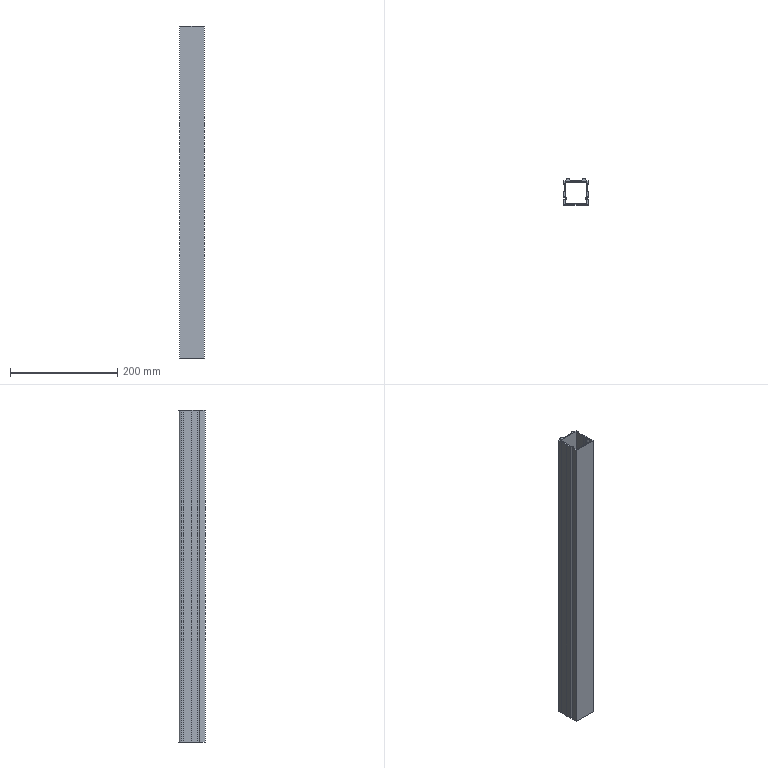Part | STEP file | MJ45 slide rail | 1 solid | 40 faces | box 45 x 49 x 620 mm | volume 255112 mm3 | plane 32 | cylinder 8 | commonest cylinder face diameters 5 x3 9 x3 8 x2
STEP:
#1=CARTESIAN_POINT('',(20.5,-14.031,310.));
#2=VERTEX_POINT('',#1);
#3=CARTESIAN_POINT('',(18.,-10.,310.));
#4=VERTEX_POINT('',#3);
#5=CARTESIAN_POINT('',(22.5,-10.,310.));
#6=DIRECTION('',(0.,0.,-1.));
#7=DIRECTION('',(1.,0.,0.));
#8=AXIS2_PLACEMENT_3D('',#5,#6,#7);
#9=CIRCLE('',#8,4.5);
#10=EDGE_CURVE('',#2,#4,#9,.T.);
#11=ORIENTED_EDGE('',*,*,#10,.T.);
#12=CARTESIAN_POINT('',(18.,-10.,-310.));
#13=VERTEX_POINT('',#12);
#14=CARTESIAN_POINT('',(18.,-10.,310.));
#15=DIRECTION('',(0.,0.,-1.));
#16=VECTOR('',#15,1000.);
#17=LINE('',#14,#16);
#18=EDGE_CURVE('',#4,#13,#17,.T.);
#19=ORIENTED_EDGE('',*,*,#18,.T.);
#20=CARTESIAN_POINT('',(20.5,-14.031,-310.));
#21=VERTEX_POINT('',#20);
#22=CARTESIAN_POINT('',(22.5,-10.,-310.));
#23=DIRECTION('',(0.,0.,-1.));
#24=DIRECTION('',(1.,0.,0.));
#25=AXIS2_PLACEMENT_3D('',#22,#23,#24);
#26=CIRCLE('',#25,4.5);
#27=EDGE_CURVE('',#21,#13,#26,.T.);
#28=ORIENTED_EDGE('',*,*,#27,.F.);
#29=CARTESIAN_POINT('',(20.5,-14.031,310.));
#30=DIRECTION('',(0.,0.,-1.));
#31=VECTOR('',#30,1000.);
#32=LINE('',#29,#31);
#33=EDGE_CURVE('',#2,#21,#32,.T.);
#34=ORIENTED_EDGE('',*,*,#33,.F.);
#35=EDGE_LOOP('',(#11,#19,#28,#34));
#36=FACE_OUTER_BOUND('',#35,.T.);
#37=CARTESIAN_POINT('',(22.5,-10.,310.));
#38=DIRECTION('',(0.,0.,-1.));
#39=DIRECTION('',(-1.,0.,0.));
#40=AXIS2_PLACEMENT_3D('',#37,#38,#39);
#41=CYLINDRICAL_SURFACE('',#40,4.5);
#42=ADVANCED_FACE('',(#36),#41,.T.);
#43=CARTESIAN_POINT('',(20.,-10.,310.));
#44=VERTEX_POINT('',#43);
#45=CARTESIAN_POINT('',(22.5,-7.5,310.));
#46=VERTEX_POINT('',#45);
#47=CARTESIAN_POINT('',(22.5,-10.,310.));
#48=DIRECTION('',(0.,0.,-1.));
#49=DIRECTION('',(1.,0.,0.));
#50=AXIS2_PLACEMENT_3D('',#47,#48,#49);
#51=CIRCLE('',#50,2.5);
#52=EDGE_CURVE('',#44,#46,#51,.T.);
#53=ORIENTED_EDGE('',*,*,#52,.F.);
#54=CARTESIAN_POINT('',(20.,-10.,-310.));
#55=VERTEX_POINT('',#54);
#56=CARTESIAN_POINT('',(20.,-10.,310.));
#57=DIRECTION('',(0.,0.,-1.));
#58=VECTOR('',#57,1000.);
#59=LINE('',#56,#58);
#60=EDGE_CURVE('',#44,#55,#59,.T.);
#61=ORIENTED_EDGE('',*,*,#60,.T.);
#62=CARTESIAN_POINT('',(22.5,-7.5,-310.));
#63=VERTEX_POINT('',#62);
#64=CARTESIAN_POINT('',(22.5,-10.,-310.));
#65=DIRECTION('',(0.,0.,-1.));
#66=DIRECTION('',(1.,0.,0.));
#67=AXIS2_PLACEMENT_3D('',#64,#65,#66);
#68=CIRCLE('',#67,2.5);
#69=EDGE_CURVE('',#55,#63,#68,.T.);
#70=ORIENTED_EDGE('',*,*,#69,.T.);
#71=CARTESIAN_POINT('',(22.5,-7.5,310.));
#72=DIRECTION('',(0.,0.,-1.));
#73=VECTOR('',#72,1000.);
#74=LINE('',#71,#73);
#75=EDGE_CURVE('',#46,#63,#74,.T.);
#76=ORIENTED_EDGE('',*,*,#75,.F.);
#77=EDGE_LOOP('',(#53,#61,#70,#76));
#78=FACE_OUTER_BOUND('',#77,.T.);
#79=CARTESIAN_POINT('',(22.5,-10.,310.));
#80=DIRECTION('',(0.,0.,-1.));
#81=DIRECTION('',(-1.,0.,0.));
#82=AXIS2_PLACEMENT_3D('',#79,#80,#81);
#83=CYLINDRICAL_SURFACE('',#82,2.5);
#84=ADVANCED_FACE('',(#78),#83,.F.);
#85=CARTESIAN_POINT('',(22.5,22.5,-310.));
#86=VERTEX_POINT('',#85);
#87=CARTESIAN_POINT('',(19.,22.5,-310.));
#88=VERTEX_POINT('',#87);
#89=CARTESIAN_POINT('',(19.,22.5,-310.));
#90=DIRECTION('',(-1.,0.,0.));
#91=VECTOR('',#90,1000.);
#92=LINE('',#89,#91);
#93=EDGE_CURVE('',#86,#88,#92,.T.);
#94=ORIENTED_EDGE('',*,*,#93,.T.);
#95=CARTESIAN_POINT('',(19.,22.5,310.));
#96=VERTEX_POINT('',#95);
#97=CARTESIAN_POINT('',(19.,22.5,310.));
#98=DIRECTION('',(0.,0.,-1.));
#99=VECTOR('',#98,1000.);
#100=LINE('',#97,#99);
#101=EDGE_CURVE('',#96,#88,#100,.T.);
#102=ORIENTED_EDGE('',*,*,#101,.F.);
#103=CARTESIAN_POINT('',(22.5,22.5,310.));
#104=VERTEX_POINT('',#103);
#105=CARTESIAN_POINT('',(19.,22.5,310.));
#106=DIRECTION('',(-1.,0.,0.));
#107=VECTOR('',#106,1000.);
#108=LINE('',#105,#107);
#109=EDGE_CURVE('',#104,#96,#108,.T.);
#110=ORIENTED_EDGE('',*,*,#109,.F.);
#111=CARTESIAN_POINT('',(22.5,22.5,310.));
#112=DIRECTION('',(0.,0.,-1.));
#113=VECTOR('',#112,1000.);
#114=LINE('',#111,#113);
#115=EDGE_CURVE('',#104,#86,#114,.T.);
#116=ORIENTED_EDGE('',*,*,#115,.T.);
#117=EDGE_LOOP('',(#94,#102,#110,#116));
#118=FACE_OUTER_BOUND('',#117,.T.);
#119=CARTESIAN_POINT('',(19.,22.5,310.));
#120=DIRECTION('',(0.,-1.,0.));
#121=DIRECTION('',(0.,0.,-1.));
#122=AXIS2_PLACEMENT_3D('',#119,#120,#121);
#123=PLANE('',#122);
#124=ADVANCED_FACE('',(#118),#123,.F.);
#125=CARTESIAN_POINT('',(11.,22.5,-310.));
#126=VERTEX_POINT('',#125);
#127=CARTESIAN_POINT('',(15.,22.5,-310.));
#128=DIRECTION('',(0.,0.,1.));
#129=DIRECTION('',(1.,0.,0.));
#130=AXIS2_PLACEMENT_3D('',#127,#128,#129);
#131=CIRCLE('',#130,4.);
#132=EDGE_CURVE('',#88,#126,#131,.T.);
#133=ORIENTED_EDGE('',*,*,#132,.T.);
#134=CARTESIAN_POINT('',(11.,22.5,310.));
#135=VERTEX_POINT('',#134);
#136=CARTESIAN_POINT('',(11.,22.5,310.));
#137=DIRECTION('',(0.,0.,-1.));
#138=VECTOR('',#137,1000.);
#139=LINE('',#136,#138);
#140=EDGE_CURVE('',#135,#126,#139,.T.);
#141=ORIENTED_EDGE('',*,*,#140,.F.);
#142=CARTESIAN_POINT('',(15.,22.5,310.));
#143=DIRECTION('',(0.,0.,1.));
#144=DIRECTION('',(1.,0.,0.));
#145=AXIS2_PLACEMENT_3D('',#142,#143,#144);
#146=CIRCLE('',#145,4.);
#147=EDGE_CURVE('',#96,#135,#146,.T.);
#148=ORIENTED_EDGE('',*,*,#147,.F.);
#149=ORIENTED_EDGE('',*,*,#101,.T.);
#150=EDGE_LOOP('',(#133,#141,#148,#149));
#151=FACE_OUTER_BOUND('',#150,.T.);
#152=CARTESIAN_POINT('',(15.,22.5,310.));
#153=DIRECTION('',(0.,0.,-1.));
#154=DIRECTION('',(-1.,0.,0.));
#155=AXIS2_PLACEMENT_3D('',#152,#153,#154);
#156=CYLINDRICAL_SURFACE('',#155,4.);
#157=ADVANCED_FACE('',(#151),#156,.T.);
#158=CARTESIAN_POINT('',(-11.,22.5,-310.));
#159=VERTEX_POINT('',#158);
#160=CARTESIAN_POINT('',(-11.,22.5,-310.));
#161=DIRECTION('',(-1.,0.,0.));
#162=VECTOR('',#161,1000.);
#163=LINE('',#160,#162);
#164=EDGE_CURVE('',#126,#159,#163,.T.);
#165=ORIENTED_EDGE('',*,*,#164,.T.);
#166=CARTESIAN_POINT('',(-11.,22.5,310.));
#167=VERTEX_POINT('',#166);
#168=CARTESIAN_POINT('',(-11.,22.5,310.));
#169=DIRECTION('',(0.,0.,-1.));
#170=VECTOR('',#169,1000.);
#171=LINE('',#168,#170);
#172=EDGE_CURVE('',#167,#159,#171,.T.);
#173=ORIENTED_EDGE('',*,*,#172,.F.);
#174=CARTESIAN_POINT('',(-11.,22.5,310.));
#175=DIRECTION('',(-1.,0.,0.));
#176=VECTOR('',#175,1000.);
#177=LINE('',#174,#176);
#178=EDGE_CURVE('',#135,#167,#177,.T.);
#179=ORIENTED_EDGE('',*,*,#178,.F.);
#180=ORIENTED_EDGE('',*,*,#140,.T.);
#181=EDGE_LOOP('',(#165,#173,#179,#180));
#182=FACE_OUTER_BOUND('',#181,.T.);
#183=CARTESIAN_POINT('',(-11.,22.5,310.));
#184=DIRECTION('',(0.,-1.,0.));
#185=DIRECTION('',(0.,0.,-1.));
#186=AXIS2_PLACEMENT_3D('',#183,#184,#185);
#187=PLANE('',#186);
#188=ADVANCED_FACE('',(#182),#187,.F.);
#189=CARTESIAN_POINT('',(-19.,22.5,-310.));
#190=VERTEX_POINT('',#189);
#191=CARTESIAN_POINT('',(-15.,22.5,-310.));
#192=DIRECTION('',(0.,0.,1.));
#193=DIRECTION('',(-1.,0.,0.));
#194=AXIS2_PLACEMENT_3D('',#191,#192,#193);
#195=CIRCLE('',#194,4.);
#196=EDGE_CURVE('',#159,#190,#195,.T.);
#197=ORIENTED_EDGE('',*,*,#196,.T.);
#198=CARTESIAN_POINT('',(-19.,22.5,310.));
#199=VERTEX_POINT('',#198);
#200=CARTESIAN_POINT('',(-19.,22.5,310.));
#201=DIRECTION('',(0.,0.,-1.));
#202=VECTOR('',#201,1000.);
#203=LINE('',#200,#202);
#204=EDGE_CURVE('',#199,#190,#203,.T.);
#205=ORIENTED_EDGE('',*,*,#204,.F.);
#206=CARTESIAN_POINT('',(-15.,22.5,310.));
#207=DIRECTION('',(0.,0.,1.));
#208=DIRECTION('',(-1.,0.,0.));
#209=AXIS2_PLACEMENT_3D('',#206,#207,#208);
#210=CIRCLE('',#209,4.);
#211=EDGE_CURVE('',#167,#199,#210,.T.);
#212=ORIENTED_EDGE('',*,*,#211,.F.);
#213=ORIENTED_EDGE('',*,*,#172,.T.);
#214=EDGE_LOOP('',(#197,#205,#212,#213));
#215=FACE_OUTER_BOUND('',#214,.T.);
#216=CARTESIAN_POINT('',(-15.,22.5,310.));
#217=DIRECTION('',(0.,0.,-1.));
#218=DIRECTION('',(-1.,0.,0.));
#219=AXIS2_PLACEMENT_3D('',#216,#217,#218);
#220=CYLINDRICAL_SURFACE('',#219,4.);
#221=ADVANCED_FACE('',(#215),#220,.T.);
#222=CARTESIAN_POINT('',(-22.5,22.5,-310.));
#223=VERTEX_POINT('',#222);
#224=CARTESIAN_POINT('',(-19.,22.5,-310.));
#225=DIRECTION('',(-1.,0.,0.));
#226=VECTOR('',#225,1000.);
#227=LINE('',#224,#226);
#228=EDGE_CURVE('',#190,#223,#227,.T.);
#229=ORIENTED_EDGE('',*,*,#228,.T.);
#230=CARTESIAN_POINT('',(-22.5,22.5,310.));
#231=VERTEX_POINT('',#230);
#232=CARTESIAN_POINT('',(-22.5,22.5,310.));
#233=DIRECTION('',(0.,0.,-1.));
#234=VECTOR('',#233,1000.);
#235=LINE('',#232,#234);
#236=EDGE_CURVE('',#231,#223,#235,.T.);
#237=ORIENTED_EDGE('',*,*,#236,.F.);
#238=CARTESIAN_POINT('',(-19.,22.5,310.));
#239=DIRECTION('',(-1.,0.,0.));
#240=VECTOR('',#239,1000.);
#241=LINE('',#238,#240);
#242=EDGE_CURVE('',#199,#231,#241,.T.);
#243=ORIENTED_EDGE('',*,*,#242,.F.);
#244=ORIENTED_EDGE('',*,*,#204,.T.);
#245=EDGE_LOOP('',(#229,#237,#243,#244));
#246=FACE_OUTER_BOUND('',#245,.T.);
#247=CARTESIAN_POINT('',(-19.,22.5,310.));
#248=DIRECTION('',(0.,-1.,0.));
#249=DIRECTION('',(1.,0.,0.));
#250=AXIS2_PLACEMENT_3D('',#247,#248,#249);
#251=PLANE('',#250);
#252=ADVANCED_FACE('',(#246),#251,.F.);
#253=CARTESIAN_POINT('',(-22.5,17.,-310.));
#254=VERTEX_POINT('',#253);
#255=CARTESIAN_POINT('',(-22.5,17.,-310.));
#256=DIRECTION('',(0.,-1.,0.));
#257=VECTOR('',#256,1000.);
#258=LINE('',#255,#257);
#259=EDGE_CURVE('',#223,#254,#258,.T.);
#260=ORIENTED_EDGE('',*,*,#259,.T.);
#261=CARTESIAN_POINT('',(-22.5,17.,310.));
#262=VERTEX_POINT('',#261);
#263=CARTESIAN_POINT('',(-22.5,17.,310.));
#264=DIRECTION('',(0.,0.,-1.));
#265=VECTOR('',#264,1000.);
#266=LINE('',#263,#265);
#267=EDGE_CURVE('',#262,#254,#266,.T.);
#268=ORIENTED_EDGE('',*,*,#267,.F.);
#269=CARTESIAN_POINT('',(-22.5,17.,310.));
#270=DIRECTION('',(0.,-1.,0.));
#271=VECTOR('',#270,1000.);
#272=LINE('',#269,#271);
#273=EDGE_CURVE('',#231,#262,#272,.T.);
#274=ORIENTED_EDGE('',*,*,#273,.F.);
#275=ORIENTED_EDGE('',*,*,#236,.T.);
#276=EDGE_LOOP('',(#260,#268,#274,#275));
#277=FACE_OUTER_BOUND('',#276,.T.);
#278=CARTESIAN_POINT('',(-22.5,17.,310.));
#279=DIRECTION('',(1.,0.,0.));
#280=DIRECTION('',(0.,1.,0.));
#281=AXIS2_PLACEMENT_3D('',#278,#279,#280);
#282=PLANE('',#281);
#283=ADVANCED_FACE('',(#277),#282,.F.);
#284=CARTESIAN_POINT('',(-21.5,17.,-310.));
#285=VERTEX_POINT('',#284);
#286=CARTESIAN_POINT('',(-21.5,17.,-310.));
#287=DIRECTION('',(1.,0.,0.));
#288=VECTOR('',#287,1000.);
#289=LINE('',#286,#288);
#290=EDGE_CURVE('',#254,#285,#289,.T.);
#291=ORIENTED_EDGE('',*,*,#290,.T.);
#292=CARTESIAN_POINT('',(-21.5,17.,310.));
#293=VERTEX_POINT('',#292);
#294=CARTESIAN_POINT('',(-21.5,17.,310.));
#295=DIRECTION('',(0.,0.,-1.));
#296=VECTOR('',#295,1000.);
#297=LINE('',#294,#296);
#298=EDGE_CURVE('',#293,#285,#297,.T.);
#299=ORIENTED_EDGE('',*,*,#298,.F.);
#300=CARTESIAN_POINT('',(-21.5,17.,310.));
#301=DIRECTION('',(1.,0.,0.));
#302=VECTOR('',#301,1000.);
#303=LINE('',#300,#302);
#304=EDGE_CURVE('',#262,#293,#303,.T.);
#305=ORIENTED_EDGE('',*,*,#304,.F.);
#306=ORIENTED_EDGE('',*,*,#267,.T.);
#307=EDGE_LOOP('',(#291,#299,#305,#306));
#308=FACE_OUTER_BOUND('',#307,.T.);
#309=CARTESIAN_POINT('',(-21.5,17.,310.));
#310=DIRECTION('',(0.,1.,0.));
#311=DIRECTION('',(0.,0.,1.));
#312=AXIS2_PLACEMENT_3D('',#309,#310,#311);
#313=PLANE('',#312);
#314=ADVANCED_FACE('',(#308),#313,.F.);
#315=CARTESIAN_POINT('',(-21.5,2.,-310.));
#316=VERTEX_POINT('',#315);
#317=CARTESIAN_POINT('',(-21.5,2.,-310.));
#318=DIRECTION('',(0.,-1.,0.));
#319=VECTOR('',#318,1000.);
#320=LINE('',#317,#319);
#321=EDGE_CURVE('',#285,#316,#320,.T.);
#322=ORIENTED_EDGE('',*,*,#321,.T.);
#323=CARTESIAN_POINT('',(-21.5,2.,310.));
#324=VERTEX_POINT('',#323);
#325=CARTESIAN_POINT('',(-21.5,2.,310.));
#326=DIRECTION('',(0.,0.,-1.));
#327=VECTOR('',#326,1000.);
#328=LINE('',#325,#327);
#329=EDGE_CURVE('',#324,#316,#328,.T.);
#330=ORIENTED_EDGE('',*,*,#329,.F.);
#331=CARTESIAN_POINT('',(-21.5,2.,310.));
#332=DIRECTION('',(0.,-1.,0.));
#333=VECTOR('',#332,1000.);
#334=LINE('',#331,#333);
#335=EDGE_CURVE('',#293,#324,#334,.T.);
#336=ORIENTED_EDGE('',*,*,#335,.F.);
#337=ORIENTED_EDGE('',*,*,#298,.T.);
#338=EDGE_LOOP('',(#322,#330,#336,#337));
#339=FACE_OUTER_BOUND('',#338,.T.);
#340=CARTESIAN_POINT('',(-21.5,2.,310.));
#341=DIRECTION('',(1.,0.,0.));
#342=DIRECTION('',(0.,0.,-1.));
#343=AXIS2_PLACEMENT_3D('',#340,#341,#342);
#344=PLANE('',#343);
#345=ADVANCED_FACE('',(#339),#344,.F.);
#346=CARTESIAN_POINT('',(-22.5,2.,-310.));
#347=VERTEX_POINT('',#346);
#348=CARTESIAN_POINT('',(-21.5,2.,-310.));
#349=DIRECTION('',(-1.,0.,0.));
#350=VECTOR('',#349,1000.);
#351=LINE('',#348,#350);
#352=EDGE_CURVE('',#316,#347,#351,.T.);
#353=ORIENTED_EDGE('',*,*,#352,.T.);
#354=CARTESIAN_POINT('',(-22.5,2.,310.));
#355=VERTEX_POINT('',#354);
#356=CARTESIAN_POINT('',(-22.5,2.,310.));
#357=DIRECTION('',(0.,0.,-1.));
#358=VECTOR('',#357,1000.);
#359=LINE('',#356,#358);
#360=EDGE_CURVE('',#355,#347,#359,.T.);
#361=ORIENTED_EDGE('',*,*,#360,.F.);
#362=CARTESIAN_POINT('',(-21.5,2.,310.));
#363=DIRECTION('',(-1.,0.,0.));
#364=VECTOR('',#363,1000.);
#365=LINE('',#362,#364);
#366=EDGE_CURVE('',#324,#355,#365,.T.);
#367=ORIENTED_EDGE('',*,*,#366,.F.);
#368=ORIENTED_EDGE('',*,*,#329,.T.);
#369=EDGE_LOOP('',(#353,#361,#367,#368));
#370=FACE_OUTER_BOUND('',#369,.T.);
#371=CARTESIAN_POINT('',(-21.5,2.,310.));
#372=DIRECTION('',(0.,-1.,0.));
#373=DIRECTION('',(0.,0.,-1.));
#374=AXIS2_PLACEMENT_3D('',#371,#372,#373);
#375=PLANE('',#374);
#376=ADVANCED_FACE('',(#370),#375,.F.);
#377=CARTESIAN_POINT('',(-22.5,-7.5,-310.));
#378=VERTEX_POINT('',#377);
#379=CARTESIAN_POINT('',(-22.5,-7.5,-310.));
#380=DIRECTION('',(0.,-1.,0.));
#381=VECTOR('',#380,1000.);
#382=LINE('',#379,#381);
#383=EDGE_CURVE('',#347,#378,#382,.T.);
#384=ORIENTED_EDGE('',*,*,#383,.T.);
#385=CARTESIAN_POINT('',(-22.5,-7.5,310.));
#386=VERTEX_POINT('',#385);
#387=CARTESIAN_POINT('',(-22.5,-7.5,310.));
#388=DIRECTION('',(0.,0.,-1.));
#389=VECTOR('',#388,1000.);
#390=LINE('',#387,#389);
#391=EDGE_CURVE('',#386,#378,#390,.T.);
#392=ORIENTED_EDGE('',*,*,#391,.F.);
#393=CARTESIAN_POINT('',(-22.5,-7.5,310.));
#394=DIRECTION('',(0.,-1.,0.));
#395=VECTOR('',#394,1000.);
#396=LINE('',#393,#395);
#397=EDGE_CURVE('',#355,#386,#396,.T.);
#398=ORIENTED_EDGE('',*,*,#397,.F.);
#399=ORIENTED_EDGE('',*,*,#360,.T.);
#400=EDGE_LOOP('',(#384,#392,#398,#399));
#401=FACE_OUTER_BOUND('',#400,.T.);
#402=CARTESIAN_POINT('',(-22.5,-7.5,310.));
#403=DIRECTION('',(1.,0.,0.));
#404=DIRECTION('',(0.,1.,0.));
#405=AXIS2_PLACEMENT_3D('',#402,#403,#404);
#406=PLANE('',#405);
#407=ADVANCED_FACE('',(#401),#406,.F.);
#408=CARTESIAN_POINT('',(-22.5,-12.5,-310.));
#409=VERTEX_POINT('',#408);
#410=CARTESIAN_POINT('',(-22.5,-10.,-310.));
#411=DIRECTION('',(0.,0.,-1.));
#412=DIRECTION('',(-1.,0.,0.));
#413=AXIS2_PLACEMENT_3D('',#410,#411,#412);
#414=CIRCLE('',#413,2.5);
#415=EDGE_CURVE('',#378,#409,#414,.T.);
#416=ORIENTED_EDGE('',*,*,#415,.T.);
#417=CARTESIAN_POINT('',(-22.5,-12.5,310.));
#418=VERTEX_POINT('',#417);
#419=CARTESIAN_POINT('',(-22.5,-12.5,310.));
#420=DIRECTION('',(0.,0.,-1.));
#421=VECTOR('',#420,1000.);
#422=LINE('',#419,#421);
#423=EDGE_CURVE('',#418,#409,#422,.T.);
#424=ORIENTED_EDGE('',*,*,#423,.F.);
#425=CARTESIAN_POINT('',(-22.5,-10.,310.));
#426=DIRECTION('',(0.,0.,-1.));
#427=DIRECTION('',(-1.,0.,0.));
#428=AXIS2_PLACEMENT_3D('',#425,#426,#427);
#429=CIRCLE('',#428,2.5);
#430=EDGE_CURVE('',#386,#418,#429,.T.);
#431=ORIENTED_EDGE('',*,*,#430,.F.);
#432=ORIENTED_EDGE('',*,*,#391,.T.);
#433=EDGE_LOOP('',(#416,#424,#431,#432));
#434=FACE_OUTER_BOUND('',#433,.T.);
#435=CARTESIAN_POINT('',(-22.5,-10.,310.));
#436=DIRECTION('',(0.,0.,-1.));
#437=DIRECTION('',(-1.,0.,0.));
#438=AXIS2_PLACEMENT_3D('',#435,#436,#437);
#439=CYLINDRICAL_SURFACE('',#438,2.5);
#440=ADVANCED_FACE('',(#434),#439,.F.);
#441=CARTESIAN_POINT('',(-22.5,-22.5,-310.));
#442=VERTEX_POINT('',#441);
#443=CARTESIAN_POINT('',(-22.5,-22.5,-310.));
#444=DIRECTION('',(0.,-1.,0.));
#445=VECTOR('',#444,1000.);
#446=LINE('',#443,#445);
#447=EDGE_CURVE('',#409,#442,#446,.T.);
#448=ORIENTED_EDGE('',*,*,#447,.T.);
#449=CARTESIAN_POINT('',(-22.5,-22.5,310.));
#450=VERTEX_POINT('',#449);
#451=CARTESIAN_POINT('',(-22.5,-22.5,310.));
#452=DIRECTION('',(0.,0.,-1.));
#453=VECTOR('',#452,1000.);
#454=LINE('',#451,#453);
#455=EDGE_CURVE('',#450,#442,#454,.T.);
#456=ORIENTED_EDGE('',*,*,#455,.F.);
#457=CARTESIAN_POINT('',(-22.5,-22.5,310.));
#458=DIRECTION('',(0.,-1.,0.));
#459=VECTOR('',#458,1000.);
#460=LINE('',#457,#459);
#461=EDGE_CURVE('',#418,#450,#460,.T.);
#462=ORIENTED_EDGE('',*,*,#461,.F.);
#463=ORIENTED_EDGE('',*,*,#423,.T.);
#464=EDGE_LOOP('',(#448,#456,#462,#463));
#465=FACE_OUTER_BOUND('',#464,.T.);
#466=CARTESIAN_POINT('',(-22.5,-22.5,310.));
#467=DIRECTION('',(1.,0.,0.));
#468=DIRECTION('',(0.,1.,0.));
#469=AXIS2_PLACEMENT_3D('',#466,#467,#468);
#470=PLANE('',#469);
#471=ADVANCED_FACE('',(#465),#470,.F.);
#472=CARTESIAN_POINT('',(22.5,-22.5,-310.));
#473=VERTEX_POINT('',#472);
#474=CARTESIAN_POINT('',(-22.5,-22.5,-310.));
#475=DIRECTION('',(1.,0.,0.));
#476=VECTOR('',#475,1000.);
#477=LINE('',#474,#476);
#478=EDGE_CURVE('',#442,#473,#477,.T.);
#479=ORIENTED_EDGE('',*,*,#478,.T.);
#480=CARTESIAN_POINT('',(22.5,-22.5,310.));
#481=VERTEX_POINT('',#480);
#482=CARTESIAN_POINT('',(22.5,-22.5,310.));
#483=DIRECTION('',(0.,0.,-1.));
#484=VECTOR('',#483,1000.);
#485=LINE('',#482,#484);
#486=EDGE_CURVE('',#481,#473,#485,.T.);
#487=ORIENTED_EDGE('',*,*,#486,.F.);
#488=CARTESIAN_POINT('',(-22.5,-22.5,310.));
#489=DIRECTION('',(1.,0.,0.));
#490=VECTOR('',#489,1000.);
#491=LINE('',#488,#490);
#492=EDGE_CURVE('',#450,#481,#491,.T.);
#493=ORIENTED_EDGE('',*,*,#492,.F.);
#494=ORIENTED_EDGE('',*,*,#455,.T.);
#495=EDGE_LOOP('',(#479,#487,#493,#494));
#496=FACE_OUTER_BOUND('',#495,.T.);
#497=CARTESIAN_POINT('',(-22.5,-22.5,310.));
#498=DIRECTION('',(0.,1.,0.));
#499=DIRECTION('',(-1.,0.,0.));
#500=AXIS2_PLACEMENT_3D('',#497,#498,#499);
#501=PLANE('',#500);
#502=ADVANCED_FACE('',(#496),#501,.F.);
#503=CARTESIAN_POINT('',(22.5,-12.5,-310.));
#504=VERTEX_POINT('',#503);
#505=CARTESIAN_POINT('',(22.5,-22.5,-310.));
#506=DIRECTION('',(0.,1.,0.));
#507=VECTOR('',#506,1000.);
#508=LINE('',#505,#507);
#509=EDGE_CURVE('',#473,#504,#508,.T.);
#510=ORIENTED_EDGE('',*,*,#509,.T.);
#511=CARTESIAN_POINT('',(22.5,-12.5,310.));
#512=VERTEX_POINT('',#511);
#513=CARTESIAN_POINT('',(22.5,-12.5,310.));
#514=DIRECTION('',(0.,0.,-1.));
#515=VECTOR('',#514,1000.);
#516=LINE('',#513,#515);
#517=EDGE_CURVE('',#512,#504,#516,.T.);
#518=ORIENTED_EDGE('',*,*,#517,.F.);
#519=CARTESIAN_POINT('',(22.5,-22.5,310.));
#520=DIRECTION('',(0.,1.,0.));
#521=VECTOR('',#520,1000.);
#522=LINE('',#519,#521);
#523=EDGE_CURVE('',#481,#512,#522,.T.);
#524=ORIENTED_EDGE('',*,*,#523,.F.);
#525=ORIENTED_EDGE('',*,*,#486,.T.);
#526=EDGE_LOOP('',(#510,#518,#524,#525));
#527=FACE_OUTER_BOUND('',#526,.T.);
#528=CARTESIAN_POINT('',(22.5,-22.5,310.));
#529=DIRECTION('',(-1.,0.,0.));
#530=DIRECTION('',(0.,-1.,0.));
#531=AXIS2_PLACEMENT_3D('',#528,#529,#530);
#532=PLANE('',#531);
#533=ADVANCED_FACE('',(#527),#532,.F.);
#534=ORIENTED_EDGE('',*,*,#60,.F.);
#535=CARTESIAN_POINT('',(22.5,-10.,310.));
#536=DIRECTION('',(0.,0.,-1.));
#537=DIRECTION('',(1.,0.,0.));
#538=AXIS2_PLACEMENT_3D('',#535,#536,#537);
#539=CIRCLE('',#538,2.5);
#540=EDGE_CURVE('',#512,#44,#539,.T.);
#541=ORIENTED_EDGE('',*,*,#540,.F.);
#542=ORIENTED_EDGE('',*,*,#517,.T.);
#543=CARTESIAN_POINT('',(22.5,-10.,-310.));
#544=DIRECTION('',(0.,0.,-1.));
#545=DIRECTION('',(1.,0.,0.));
#546=AXIS2_PLACEMENT_3D('',#543,#544,#545);
#547=CIRCLE('',#546,2.5);
#548=EDGE_CURVE('',#504,#55,#547,.T.);
#549=ORIENTED_EDGE('',*,*,#548,.T.);
#550=EDGE_LOOP('',(#534,#541,#542,#549));
#551=FACE_OUTER_BOUND('',#550,.T.);
#552=CARTESIAN_POINT('',(22.5,-10.,310.));
#553=DIRECTION('',(0.,0.,-1.));
#554=DIRECTION('',(-1.,0.,0.));
#555=AXIS2_PLACEMENT_3D('',#552,#553,#554);
#556=CYLINDRICAL_SURFACE('',#555,2.5);
#557=ADVANCED_FACE('',(#551),#556,.F.);
#558=CARTESIAN_POINT('',(22.5,2.,-310.));
#559=VERTEX_POINT('',#558);
#560=CARTESIAN_POINT('',(22.5,-7.5,-310.));
#561=DIRECTION('',(0.,1.,0.));
#562=VECTOR('',#561,1000.);
#563=LINE('',#560,#562);
#564=EDGE_CURVE('',#63,#559,#563,.T.);
#565=ORIENTED_EDGE('',*,*,#564,.T.);
#566=CARTESIAN_POINT('',(22.5,2.,310.));
#567=VERTEX_POINT('',#566);
#568=CARTESIAN_POINT('',(22.5,2.,310.));
#569=DIRECTION('',(0.,0.,-1.));
#570=VECTOR('',#569,1000.);
#571=LINE('',#568,#570);
#572=EDGE_CURVE('',#567,#559,#571,.T.);
#573=ORIENTED_EDGE('',*,*,#572,.F.);
#574=CARTESIAN_POINT('',(22.5,-7.5,310.));
#575=DIRECTION('',(0.,1.,0.));
#576=VECTOR('',#575,1000.);
#577=LINE('',#574,#576);
#578=EDGE_CURVE('',#46,#567,#577,.T.);
#579=ORIENTED_EDGE('',*,*,#578,.F.);
#580=ORIENTED_EDGE('',*,*,#75,.T.);
#581=EDGE_LOOP('',(#565,#573,#579,#580));
#582=FACE_OUTER_BOUND('',#581,.T.);
#583=CARTESIAN_POINT('',(22.5,-7.5,310.));
#584=DIRECTION('',(-1.,0.,0.));
#585=DIRECTION('',(0.,0.,1.));
#586=AXIS2_PLACEMENT_3D('',#583,#584,#585);
#587=PLANE('',#586);
#588=ADVANCED_FACE('',(#582),#587,.F.);
#589=CARTESIAN_POINT('',(21.5,2.,-310.));
#590=VERTEX_POINT('',#589);
#591=CARTESIAN_POINT('',(21.5,2.,-310.));
#592=DIRECTION('',(-1.,0.,0.));
#593=VECTOR('',#592,1000.);
#594=LINE('',#591,#593);
#595=EDGE_CURVE('',#559,#590,#594,.T.);
#596=ORIENTED_EDGE('',*,*,#595,.T.);
#597=CARTESIAN_POINT('',(21.5,2.,310.));
#598=VERTEX_POINT('',#597);
#599=CARTESIAN_POINT('',(21.5,2.,310.));
#600=DIRECTION('',(0.,0.,-1.));
#601=VECTOR('',#600,1000.);
#602=LINE('',#599,#601);
#603=EDGE_CURVE('',#598,#590,#602,.T.);
#604=ORIENTED_EDGE('',*,*,#603,.F.);
#605=CARTESIAN_POINT('',(21.5,2.,310.));
#606=DIRECTION('',(-1.,0.,0.));
#607=VECTOR('',#606,1000.);
#608=LINE('',#605,#607);
#609=EDGE_CURVE('',#567,#598,#608,.T.);
#610=ORIENTED_EDGE('',*,*,#609,.F.);
#611=ORIENTED_EDGE('',*,*,#572,.T.);
#612=EDGE_LOOP('',(#596,#604,#610,#611));
#613=FACE_OUTER_BOUND('',#612,.T.);
#614=CARTESIAN_POINT('',(21.5,2.,310.));
#615=DIRECTION('',(0.,-1.,0.));
#616=DIRECTION('',(0.,0.,-1.));
#617=AXIS2_PLACEMENT_3D('',#614,#615,#616);
#618=PLANE('',#617);
#619=ADVANCED_FACE('',(#613),#618,.F.);
#620=CARTESIAN_POINT('',(21.5,17.,-310.));
#621=VERTEX_POINT('',#620);
#622=CARTESIAN_POINT('',(21.5,2.,-310.));
#623=DIRECTION('',(0.,1.,0.));
#624=VECTOR('',#623,1000.);
#625=LINE('',#622,#624);
#626=EDGE_CURVE('',#590,#621,#625,.T.);
#627=ORIENTED_EDGE('',*,*,#626,.T.);
#628=CARTESIAN_POINT('',(21.5,17.,310.));
#629=VERTEX_POINT('',#628);
#630=CARTESIAN_POINT('',(21.5,17.,310.));
#631=DIRECTION('',(0.,0.,-1.));
#632=VECTOR('',#631,1000.);
#633=LINE('',#630,#632);
#634=EDGE_CURVE('',#629,#621,#633,.T.);
#635=ORIENTED_EDGE('',*,*,#634,.F.);
#636=CARTESIAN_POINT('',(21.5,2.,310.));
#637=DIRECTION('',(0.,1.,0.));
#638=VECTOR('',#637,1000.);
#639=LINE('',#636,#638);
#640=EDGE_CURVE('',#598,#629,#639,.T.);
#641=ORIENTED_EDGE('',*,*,#640,.F.);
#642=ORIENTED_EDGE('',*,*,#603,.T.);
#643=EDGE_LOOP('',(#627,#635,#641,#642));
#644=FACE_OUTER_BOUND('',#643,.T.);
#645=CARTESIAN_POINT('',(21.5,2.,310.));
#646=DIRECTION('',(-1.,0.,0.));
#647=DIRECTION('',(0.,0.,1.));
#648=AXIS2_PLACEMENT_3D('',#645,#646,#647);
#649=PLANE('',#648);
#650=ADVANCED_FACE('',(#644),#649,.F.);
#651=CARTESIAN_POINT('',(22.5,17.,-310.));
#652=VERTEX_POINT('',#651);
#653=CARTESIAN_POINT('',(21.5,17.,-310.));
#654=DIRECTION('',(1.,0.,0.));
#655=VECTOR('',#654,1000.);
#656=LINE('',#653,#655);
#657=EDGE_CURVE('',#621,#652,#656,.T.);
#658=ORIENTED_EDGE('',*,*,#657,.T.);
#659=CARTESIAN_POINT('',(22.5,17.,310.));
#660=VERTEX_POINT('',#659);
#661=CARTESIAN_POINT('',(22.5,17.,310.));
#662=DIRECTION('',(0.,0.,-1.));
#663=VECTOR('',#662,1000.);
#664=LINE('',#661,#663);
#665=EDGE_CURVE('',#660,#652,#664,.T.);
#666=ORIENTED_EDGE('',*,*,#665,.F.);
#667=CARTESIAN_POINT('',(21.5,17.,310.));
#668=DIRECTION('',(1.,0.,0.));
#669=VECTOR('',#668,1000.);
#670=LINE('',#667,#669);
#671=EDGE_CURVE('',#629,#660,#670,.T.);
#672=ORIENTED_EDGE('',*,*,#671,.F.);
#673=ORIENTED_EDGE('',*,*,#634,.T.);
#674=EDGE_LOOP('',(#658,#666,#672,#673));
#675=FACE_OUTER_BOUND('',#674,.T.);
#676=CARTESIAN_POINT('',(21.5,17.,310.));
#677=DIRECTION('',(0.,1.,0.));
#678=DIRECTION('',(0.,0.,1.));
#679=AXIS2_PLACEMENT_3D('',#676,#677,#678);
#680=PLANE('',#679);
#681=ADVANCED_FACE('',(#675),#680,.F.);
#682=CARTESIAN_POINT('',(22.5,17.,-310.));
#683=DIRECTION('',(0.,1.,0.));
#684=VECTOR('',#683,1000.);
#685=LINE('',#682,#684);
#686=EDGE_CURVE('',#652,#86,#685,.T.);
#687=ORIENTED_EDGE('',*,*,#686,.T.);
#688=ORIENTED_EDGE('',*,*,#115,.F.);
#689=CARTESIAN_POINT('',(22.5,17.,310.));
#690=DIRECTION('',(0.,1.,0.));
#691=VECTOR('',#690,1000.);
#692=LINE('',#689,#691);
#693=EDGE_CURVE('',#660,#104,#692,.T.);
#694=ORIENTED_EDGE('',*,*,#693,.F.);
#695=ORIENTED_EDGE('',*,*,#665,.T.);
#696=EDGE_LOOP('',(#687,#688,#694,#695));
#697=FACE_OUTER_BOUND('',#696,.T.);
#698=CARTESIAN_POINT('',(22.5,17.,310.));
#699=DIRECTION('',(-1.,0.,0.));
#700=DIRECTION('',(0.,-1.,0.));
#701=AXIS2_PLACEMENT_3D('',#698,#699,#700);
#702=PLANE('',#701);
#703=ADVANCED_FACE('',(#697),#702,.F.);
#704=CARTESIAN_POINT('',(20.5,20.5,310.));
#705=VERTEX_POINT('',#704);
#706=CARTESIAN_POINT('',(-20.5,20.5,310.));
#707=VERTEX_POINT('',#706);
#708=CARTESIAN_POINT('',(19.,20.5,310.));
#709=DIRECTION('',(-1.,0.,0.));
#710=VECTOR('',#709,1000.);
#711=LINE('',#708,#710);
#712=EDGE_CURVE('',#705,#707,#711,.T.);
#713=ORIENTED_EDGE('',*,*,#712,.F.);
#714=CARTESIAN_POINT('',(20.5,19.,310.));
#715=VERTEX_POINT('',#714);
#716=CARTESIAN_POINT('',(20.5,17.,310.));
#717=DIRECTION('',(0.,1.,0.));
#718=VECTOR('',#717,1000.);
#719=LINE('',#716,#718);
#720=EDGE_CURVE('',#715,#705,#719,.T.);
#721=ORIENTED_EDGE('',*,*,#720,.F.);
#722=CARTESIAN_POINT('',(19.5,19.,310.));
#723=VERTEX_POINT('',#722);
#724=CARTESIAN_POINT('',(21.5,19.,310.));
#725=DIRECTION('',(1.,0.,0.));
#726=VECTOR('',#725,1000.);
#727=LINE('',#724,#726);
#728=EDGE_CURVE('',#723,#715,#727,.T.);
#729=ORIENTED_EDGE('',*,*,#728,.F.);
#730=CARTESIAN_POINT('',(19.5,0.,310.));
#731=VERTEX_POINT('',#730);
#732=CARTESIAN_POINT('',(19.5,2.,310.));
#733=DIRECTION('',(0.,1.,0.));
#734=VECTOR('',#733,1000.);
#735=LINE('',#732,#734);
#736=EDGE_CURVE('',#731,#723,#735,.T.);
#737=ORIENTED_EDGE('',*,*,#736,.F.);
#738=CARTESIAN_POINT('',(20.5,0.,310.));
#739=VERTEX_POINT('',#738);
#740=CARTESIAN_POINT('',(21.5,0.,310.));
#741=DIRECTION('',(-1.,0.,0.));
#742=VECTOR('',#741,1000.);
#743=LINE('',#740,#742);
#744=EDGE_CURVE('',#739,#731,#743,.T.);
#745=ORIENTED_EDGE('',*,*,#744,.F.);
#746=CARTESIAN_POINT('',(20.5,-5.969,310.));
#747=VERTEX_POINT('',#746);
#748=CARTESIAN_POINT('',(20.5,-7.5,310.));
#749=DIRECTION('',(0.,1.,0.));
#750=VECTOR('',#749,1000.);
#751=LINE('',#748,#750);
#752=EDGE_CURVE('',#747,#739,#751,.T.);
#753=ORIENTED_EDGE('',*,*,#752,.F.);
#754=CARTESIAN_POINT('',(22.5,-10.,310.));
#755=DIRECTION('',(0.,0.,-1.));
#756=DIRECTION('',(1.,0.,0.));
#757=AXIS2_PLACEMENT_3D('',#754,#755,#756);
#758=CIRCLE('',#757,4.5);
#759=EDGE_CURVE('',#4,#747,#758,.T.);
#760=ORIENTED_EDGE('',*,*,#759,.F.);
#761=ORIENTED_EDGE('',*,*,#10,.F.);
#762=CARTESIAN_POINT('',(20.5,-20.5,310.));
#763=VERTEX_POINT('',#762);
#764=CARTESIAN_POINT('',(20.5,-22.5,310.));
#765=DIRECTION('',(0.,1.,0.));
#766=VECTOR('',#765,1000.);
#767=LINE('',#764,#766);
#768=EDGE_CURVE('',#763,#2,#767,.T.);
#769=ORIENTED_EDGE('',*,*,#768,.F.);
#770=CARTESIAN_POINT('',(-20.5,-20.5,310.));
#771=VERTEX_POINT('',#770);
#772=CARTESIAN_POINT('',(-22.5,-20.5,310.));
#773=DIRECTION('',(1.,0.,0.));
#774=VECTOR('',#773,1000.);
#775=LINE('',#772,#774);
#776=EDGE_CURVE('',#771,#763,#775,.T.);
#777=ORIENTED_EDGE('',*,*,#776,.F.);
#778=CARTESIAN_POINT('',(-20.5,-14.031,310.));
#779=VERTEX_POINT('',#778);
#780=CARTESIAN_POINT('',(-20.5,-22.5,310.));
#781=DIRECTION('',(0.,-1.,0.));
#782=VECTOR('',#781,1000.);
#783=LINE('',#780,#782);
#784=EDGE_CURVE('',#779,#771,#783,.T.);
#785=ORIENTED_EDGE('',*,*,#784,.F.);
#786=CARTESIAN_POINT('',(-20.5,-5.969,310.));
#787=VERTEX_POINT('',#786);
#788=CARTESIAN_POINT('',(-22.5,-10.,310.));
#789=DIRECTION('',(0.,0.,-1.));
#790=DIRECTION('',(1.,0.,0.));
#791=AXIS2_PLACEMENT_3D('',#788,#789,#790);
#792=CIRCLE('',#791,4.5);
#793=EDGE_CURVE('',#787,#779,#792,.T.);
#794=ORIENTED_EDGE('',*,*,#793,.F.);
#795=CARTESIAN_POINT('',(-20.5,0.,310.));
#796=VERTEX_POINT('',#795);
#797=CARTESIAN_POINT('',(-20.5,-7.5,310.));
#798=DIRECTION('',(0.,-1.,0.));
#799=VECTOR('',#798,1000.);
#800=LINE('',#797,#799);
#801=EDGE_CURVE('',#796,#787,#800,.T.);
#802=ORIENTED_EDGE('',*,*,#801,.F.);
#803=CARTESIAN_POINT('',(-19.5,0.,310.));
#804=VERTEX_POINT('',#803);
#805=CARTESIAN_POINT('',(-21.5,0.,310.));
#806=DIRECTION('',(-1.,0.,0.));
#807=VECTOR('',#806,1000.);
#808=LINE('',#805,#807);
#809=EDGE_CURVE('',#804,#796,#808,.T.);
#810=ORIENTED_EDGE('',*,*,#809,.F.);
#811=CARTESIAN_POINT('',(-19.5,19.,310.));
#812=VERTEX_POINT('',#811);
#813=CARTESIAN_POINT('',(-19.5,2.,310.));
#814=DIRECTION('',(0.,-1.,0.));
#815=VECTOR('',#814,1000.);
#816=LINE('',#813,#815);
#817=EDGE_CURVE('',#812,#804,#816,.T.);
#818=ORIENTED_EDGE('',*,*,#817,.F.);
#819=CARTESIAN_POINT('',(-20.5,19.,310.));
#820=VERTEX_POINT('',#819);
#821=CARTESIAN_POINT('',(-21.5,19.,310.));
#822=DIRECTION('',(1.,0.,0.));
#823=VECTOR('',#822,1000.);
#824=LINE('',#821,#823);
#825=EDGE_CURVE('',#820,#812,#824,.T.);
#826=ORIENTED_EDGE('',*,*,#825,.F.);
#827=CARTESIAN_POINT('',(-20.5,17.,310.));
#828=DIRECTION('',(0.,-1.,0.));
#829=VECTOR('',#828,1000.);
#830=LINE('',#827,#829);
#831=EDGE_CURVE('',#707,#820,#830,.T.);
#832=ORIENTED_EDGE('',*,*,#831,.F.);
#833=EDGE_LOOP('',(#713,#721,#729,#737,#745,#753,#760,#761,#769,#777,#785,#794,#802,#810,#818,#826,#832));
#834=FACE_BOUND('',#833,.T.);
#835=ORIENTED_EDGE('',*,*,#109,.T.);
#836=ORIENTED_EDGE('',*,*,#147,.T.);
#837=ORIENTED_EDGE('',*,*,#178,.T.);
#838=ORIENTED_EDGE('',*,*,#211,.T.);
#839=ORIENTED_EDGE('',*,*,#242,.T.);
#840=ORIENTED_EDGE('',*,*,#273,.T.);
#841=ORIENTED_EDGE('',*,*,#304,.T.);
#842=ORIENTED_EDGE('',*,*,#335,.T.);
#843=ORIENTED_EDGE('',*,*,#366,.T.);
#844=ORIENTED_EDGE('',*,*,#397,.T.);
#845=ORIENTED_EDGE('',*,*,#430,.T.);
#846=ORIENTED_EDGE('',*,*,#461,.T.);
#847=ORIENTED_EDGE('',*,*,#492,.T.);
#848=ORIENTED_EDGE('',*,*,#523,.T.);
#849=ORIENTED_EDGE('',*,*,#540,.T.);
#850=ORIENTED_EDGE('',*,*,#52,.T.);
#851=ORIENTED_EDGE('',*,*,#578,.T.);
#852=ORIENTED_EDGE('',*,*,#609,.T.);
#853=ORIENTED_EDGE('',*,*,#640,.T.);
#854=ORIENTED_EDGE('',*,*,#671,.T.);
#855=ORIENTED_EDGE('',*,*,#693,.T.);
#856=EDGE_LOOP('',(#835,#836,#837,#838,#839,#840,#841,#842,#843,#844,#845,#846,#847,#848,#849,#850,#851,#852,#853,#854,#855));
#857=FACE_OUTER_BOUND('',#856,.T.);
#858=CARTESIAN_POINT('',(22.5,-10.,310.));
#859=DIRECTION('',(0.,0.,1.));
#860=DIRECTION('',(1.,0.,0.));
#861=AXIS2_PLACEMENT_3D('',#858,#859,#860);
#862=PLANE('',#861);
#863=ADVANCED_FACE('',(#834,#857),#862,.T.);
#864=CARTESIAN_POINT('',(20.5,19.,-310.));
#865=VERTEX_POINT('',#864);
#866=CARTESIAN_POINT('',(20.5,20.5,-310.));
#867=VERTEX_POINT('',#866);
#868=CARTESIAN_POINT('',(20.5,17.,-310.));
#869=DIRECTION('',(0.,1.,0.));
#870=VECTOR('',#869,1000.);
#871=LINE('',#868,#870);
#872=EDGE_CURVE('',#865,#867,#871,.T.);
#873=ORIENTED_EDGE('',*,*,#872,.T.);
#874=CARTESIAN_POINT('',(-20.5,20.5,-310.));
#875=VERTEX_POINT('',#874);
#876=CARTESIAN_POINT('',(-19.,20.5,-310.));
#877=DIRECTION('',(-1.,0.,0.));
#878=VECTOR('',#877,1000.);
#879=LINE('',#876,#878);
#880=EDGE_CURVE('',#867,#875,#879,.T.);
#881=ORIENTED_EDGE('',*,*,#880,.T.);
#882=CARTESIAN_POINT('',(-20.5,19.,-310.));
#883=VERTEX_POINT('',#882);
#884=CARTESIAN_POINT('',(-20.5,17.,-310.));
#885=DIRECTION('',(0.,-1.,0.));
#886=VECTOR('',#885,1000.);
#887=LINE('',#884,#886);
#888=EDGE_CURVE('',#875,#883,#887,.T.);
#889=ORIENTED_EDGE('',*,*,#888,.T.);
#890=CARTESIAN_POINT('',(-19.5,19.,-310.));
#891=VERTEX_POINT('',#890);
#892=CARTESIAN_POINT('',(-21.5,19.,-310.));
#893=DIRECTION('',(1.,0.,0.));
#894=VECTOR('',#893,1000.);
#895=LINE('',#892,#894);
#896=EDGE_CURVE('',#883,#891,#895,.T.);
#897=ORIENTED_EDGE('',*,*,#896,.T.);
#898=CARTESIAN_POINT('',(-19.5,0.,-310.));
#899=VERTEX_POINT('',#898);
#900=CARTESIAN_POINT('',(-19.5,2.,-310.));
#901=DIRECTION('',(0.,-1.,0.));
#902=VECTOR('',#901,1000.);
#903=LINE('',#900,#902);
#904=EDGE_CURVE('',#891,#899,#903,.T.);
#905=ORIENTED_EDGE('',*,*,#904,.T.);
#906=CARTESIAN_POINT('',(-20.5,0.,-310.));
#907=VERTEX_POINT('',#906);
#908=CARTESIAN_POINT('',(-21.5,0.,-310.));
#909=DIRECTION('',(-1.,0.,0.));
#910=VECTOR('',#909,1000.);
#911=LINE('',#908,#910);
#912=EDGE_CURVE('',#899,#907,#911,.T.);
#913=ORIENTED_EDGE('',*,*,#912,.T.);
#914=CARTESIAN_POINT('',(-20.5,-5.969,-310.));
#915=VERTEX_POINT('',#914);
#916=CARTESIAN_POINT('',(-20.5,-7.5,-310.));
#917=DIRECTION('',(0.,-1.,0.));
#918=VECTOR('',#917,1000.);
#919=LINE('',#916,#918);
#920=EDGE_CURVE('',#907,#915,#919,.T.);
#921=ORIENTED_EDGE('',*,*,#920,.T.);
#922=CARTESIAN_POINT('',(-20.5,-14.031,-310.));
#923=VERTEX_POINT('',#922);
#924=CARTESIAN_POINT('',(-22.5,-10.,-310.));
#925=DIRECTION('',(0.,0.,-1.));
#926=DIRECTION('',(1.,0.,0.));
#927=AXIS2_PLACEMENT_3D('',#924,#925,#926);
#928=CIRCLE('',#927,4.5);
#929=EDGE_CURVE('',#915,#923,#928,.T.);
#930=ORIENTED_EDGE('',*,*,#929,.T.);
#931=CARTESIAN_POINT('',(-20.5,-20.5,-310.));
#932=VERTEX_POINT('',#931);
#933=CARTESIAN_POINT('',(-20.5,-22.5,-310.));
#934=DIRECTION('',(0.,-1.,0.));
#935=VECTOR('',#934,1000.);
#936=LINE('',#933,#935);
#937=EDGE_CURVE('',#923,#932,#936,.T.);
#938=ORIENTED_EDGE('',*,*,#937,.T.);
#939=CARTESIAN_POINT('',(20.5,-20.5,-310.));
#940=VERTEX_POINT('',#939);
#941=CARTESIAN_POINT('',(-22.5,-20.5,-310.));
#942=DIRECTION('',(1.,0.,0.));
#943=VECTOR('',#942,1000.);
#944=LINE('',#941,#943);
#945=EDGE_CURVE('',#932,#940,#944,.T.);
#946=ORIENTED_EDGE('',*,*,#945,.T.);
#947=CARTESIAN_POINT('',(20.5,-22.5,-310.));
#948=DIRECTION('',(0.,1.,0.));
#949=VECTOR('',#948,1000.);
#950=LINE('',#947,#949);
#951=EDGE_CURVE('',#940,#21,#950,.T.);
#952=ORIENTED_EDGE('',*,*,#951,.T.);
#953=ORIENTED_EDGE('',*,*,#27,.T.);
#954=CARTESIAN_POINT('',(20.5,-5.969,-310.));
#955=VERTEX_POINT('',#954);
#956=CARTESIAN_POINT('',(22.5,-10.,-310.));
#957=DIRECTION('',(0.,0.,-1.));
#958=DIRECTION('',(1.,0.,0.));
#959=AXIS2_PLACEMENT_3D('',#956,#957,#958);
#960=CIRCLE('',#959,4.5);
#961=EDGE_CURVE('',#13,#955,#960,.T.);
#962=ORIENTED_EDGE('',*,*,#961,.T.);
#963=CARTESIAN_POINT('',(20.5,0.,-310.));
#964=VERTEX_POINT('',#963);
#965=CARTESIAN_POINT('',(20.5,-7.5,-310.));
#966=DIRECTION('',(0.,1.,0.));
#967=VECTOR('',#966,1000.);
#968=LINE('',#965,#967);
#969=EDGE_CURVE('',#955,#964,#968,.T.);
#970=ORIENTED_EDGE('',*,*,#969,.T.);
#971=CARTESIAN_POINT('',(19.5,0.,-310.));
#972=VERTEX_POINT('',#971);
#973=CARTESIAN_POINT('',(21.5,0.,-310.));
#974=DIRECTION('',(-1.,0.,0.));
#975=VECTOR('',#974,1000.);
#976=LINE('',#973,#975);
#977=EDGE_CURVE('',#964,#972,#976,.T.);
#978=ORIENTED_EDGE('',*,*,#977,.T.);
#979=CARTESIAN_POINT('',(19.5,19.,-310.));
#980=VERTEX_POINT('',#979);
#981=CARTESIAN_POINT('',(19.5,2.,-310.));
#982=DIRECTION('',(0.,1.,0.));
#983=VECTOR('',#982,1000.);
#984=LINE('',#981,#983);
#985=EDGE_CURVE('',#972,#980,#984,.T.);
#986=ORIENTED_EDGE('',*,*,#985,.T.);
#987=CARTESIAN_POINT('',(21.5,19.,-310.));
#988=DIRECTION('',(1.,0.,0.));
#989=VECTOR('',#988,1000.);
#990=LINE('',#987,#989);
#991=EDGE_CURVE('',#980,#865,#990,.T.);
#992=ORIENTED_EDGE('',*,*,#991,.T.);
#993=EDGE_LOOP('',(#873,#881,#889,#897,#905,#913,#921,#930,#938,#946,#952,#953,#962,#970,#978,#986,#992));
#994=FACE_BOUND('',#993,.T.);
#995=ORIENTED_EDGE('',*,*,#93,.F.);
#996=ORIENTED_EDGE('',*,*,#686,.F.);
#997=ORIENTED_EDGE('',*,*,#657,.F.);
#998=ORIENTED_EDGE('',*,*,#626,.F.);
#999=ORIENTED_EDGE('',*,*,#595,.F.);
#1000=ORIENTED_EDGE('',*,*,#564,.F.);
#1001=ORIENTED_EDGE('',*,*,#69,.F.);
#1002=ORIENTED_EDGE('',*,*,#548,.F.);
#1003=ORIENTED_EDGE('',*,*,#509,.F.);
#1004=ORIENTED_EDGE('',*,*,#478,.F.);
#1005=ORIENTED_EDGE('',*,*,#447,.F.);
#1006=ORIENTED_EDGE('',*,*,#415,.F.);
#1007=ORIENTED_EDGE('',*,*,#383,.F.);
#1008=ORIENTED_EDGE('',*,*,#352,.F.);
#1009=ORIENTED_EDGE('',*,*,#321,.F.);
#1010=ORIENTED_EDGE('',*,*,#290,.F.);
#1011=ORIENTED_EDGE('',*,*,#259,.F.);
#1012=ORIENTED_EDGE('',*,*,#228,.F.);
#1013=ORIENTED_EDGE('',*,*,#196,.F.);
#1014=ORIENTED_EDGE('',*,*,#164,.F.);
#1015=ORIENTED_EDGE('',*,*,#132,.F.);
#1016=EDGE_LOOP('',(#995,#996,#997,#998,#999,#1000,#1001,#1002,#1003,#1004,#1005,#1006,#1007,#1008,#1009,#1010,#1011,#1012,#1013,#1014,#1015));
#1017=FACE_OUTER_BOUND('',#1016,.T.);
#1018=CARTESIAN_POINT('',(22.5,-10.,-310.));
#1019=DIRECTION('',(0.,0.,1.));
#1020=DIRECTION('',(1.,0.,0.));
#1021=AXIS2_PLACEMENT_3D('',#1018,#1019,#1020);
#1022=PLANE('',#1021);
#1023=ADVANCED_FACE('',(#994,#1017),#1022,.F.);
#1024=ORIENTED_EDGE('',*,*,#880,.F.);
#1025=CARTESIAN_POINT('',(20.5,20.5,310.));
#1026=DIRECTION('',(0.,0.,-1.));
#1027=VECTOR('',#1026,1000.);
#1028=LINE('',#1025,#1027);
#1029=EDGE_CURVE('',#705,#867,#1028,.T.);
#1030=ORIENTED_EDGE('',*,*,#1029,.F.);
#1031=ORIENTED_EDGE('',*,*,#712,.T.);
#1032=CARTESIAN_POINT('',(-20.5,20.5,310.));
#1033=DIRECTION('',(0.,0.,-1.));
#1034=VECTOR('',#1033,1000.);
#1035=LINE('',#1032,#1034);
#1036=EDGE_CURVE('',#707,#875,#1035,.T.);
#1037=ORIENTED_EDGE('',*,*,#1036,.T.);
#1038=EDGE_LOOP('',(#1024,#1030,#1031,#1037));
#1039=FACE_OUTER_BOUND('',#1038,.T.);
#1040=CARTESIAN_POINT('',(-19.,20.5,310.));
#1041=DIRECTION('',(0.,-1.,0.));
#1042=DIRECTION('',(1.,0.,0.));
#1043=AXIS2_PLACEMENT_3D('',#1040,#1041,#1042);
#1044=PLANE('',#1043);
#1045=ADVANCED_FACE('',(#1039),#1044,.T.);
#1046=ORIENTED_EDGE('',*,*,#888,.F.);
#1047=ORIENTED_EDGE('',*,*,#1036,.F.);
#1048=ORIENTED_EDGE('',*,*,#831,.T.);
#1049=CARTESIAN_POINT('',(-20.5,19.,310.));
#1050=DIRECTION('',(0.,0.,-1.));
#1051=VECTOR('',#1050,1000.);
#1052=LINE('',#1049,#1051);
#1053=EDGE_CURVE('',#820,#883,#1052,.T.);
#1054=ORIENTED_EDGE('',*,*,#1053,.T.);
#1055=EDGE_LOOP('',(#1046,#1047,#1048,#1054));
#1056=FACE_OUTER_BOUND('',#1055,.T.);
#1057=CARTESIAN_POINT('',(-20.5,17.,310.));
#1058=DIRECTION('',(1.,0.,0.));
#1059=DIRECTION('',(0.,1.,0.));
#1060=AXIS2_PLACEMENT_3D('',#1057,#1058,#1059);
#1061=PLANE('',#1060);
#1062=ADVANCED_FACE('',(#1056),#1061,.T.);
#1063=ORIENTED_EDGE('',*,*,#896,.F.);
#1064=ORIENTED_EDGE('',*,*,#1053,.F.);
#1065=ORIENTED_EDGE('',*,*,#825,.T.);
#1066=CARTESIAN_POINT('',(-19.5,19.,310.));
#1067=DIRECTION('',(0.,0.,-1.));
#1068=VECTOR('',#1067,1000.);
#1069=LINE('',#1066,#1068);
#1070=EDGE_CURVE('',#812,#891,#1069,.T.);
#1071=ORIENTED_EDGE('',*,*,#1070,.T.);
#1072=EDGE_LOOP('',(#1063,#1064,#1065,#1071));
#1073=FACE_OUTER_BOUND('',#1072,.T.);
#1074=CARTESIAN_POINT('',(-21.5,19.,310.));
#1075=DIRECTION('',(0.,1.,0.));
#1076=DIRECTION('',(0.,0.,1.));
#1077=AXIS2_PLACEMENT_3D('',#1074,#1075,#1076);
#1078=PLANE('',#1077);
#1079=ADVANCED_FACE('',(#1073),#1078,.T.);
#1080=ORIENTED_EDGE('',*,*,#904,.F.);
#1081=ORIENTED_EDGE('',*,*,#1070,.F.);
#1082=ORIENTED_EDGE('',*,*,#817,.T.);
#1083=CARTESIAN_POINT('',(-19.5,0.,310.));
#1084=DIRECTION('',(0.,0.,-1.));
#1085=VECTOR('',#1084,1000.);
#1086=LINE('',#1083,#1085);
#1087=EDGE_CURVE('',#804,#899,#1086,.T.);
#1088=ORIENTED_EDGE('',*,*,#1087,.T.);
#1089=EDGE_LOOP('',(#1080,#1081,#1082,#1088));
#1090=FACE_OUTER_BOUND('',#1089,.T.);
#1091=CARTESIAN_POINT('',(-19.5,2.,310.));
#1092=DIRECTION('',(1.,0.,0.));
#1093=DIRECTION('',(0.,0.,-1.));
#1094=AXIS2_PLACEMENT_3D('',#1091,#1092,#1093);
#1095=PLANE('',#1094);
#1096=ADVANCED_FACE('',(#1090),#1095,.T.);
#1097=ORIENTED_EDGE('',*,*,#912,.F.);
#1098=ORIENTED_EDGE('',*,*,#1087,.F.);
#1099=ORIENTED_EDGE('',*,*,#809,.T.);
#1100=CARTESIAN_POINT('',(-20.5,0.,310.));
#1101=DIRECTION('',(0.,0.,-1.));
#1102=VECTOR('',#1101,1000.);
#1103=LINE('',#1100,#1102);
#1104=EDGE_CURVE('',#796,#907,#1103,.T.);
#1105=ORIENTED_EDGE('',*,*,#1104,.T.);
#1106=EDGE_LOOP('',(#1097,#1098,#1099,#1105));
#1107=FACE_OUTER_BOUND('',#1106,.T.);
#1108=CARTESIAN_POINT('',(-21.5,0.,310.));
#1109=DIRECTION('',(0.,-1.,0.));
#1110=DIRECTION('',(0.,0.,-1.));
#1111=AXIS2_PLACEMENT_3D('',#1108,#1109,#1110);
#1112=PLANE('',#1111);
#1113=ADVANCED_FACE('',(#1107),#1112,.T.);
#1114=ORIENTED_EDGE('',*,*,#920,.F.);
#1115=ORIENTED_EDGE('',*,*,#1104,.F.);
#1116=ORIENTED_EDGE('',*,*,#801,.T.);
#1117=CARTESIAN_POINT('',(-20.5,-5.969,310.));
#1118=DIRECTION('',(0.,0.,-1.));
#1119=VECTOR('',#1118,1000.);
#1120=LINE('',#1117,#1119);
#1121=EDGE_CURVE('',#787,#915,#1120,.T.);
#1122=ORIENTED_EDGE('',*,*,#1121,.T.);
#1123=EDGE_LOOP('',(#1114,#1115,#1116,#1122));
#1124=FACE_OUTER_BOUND('',#1123,.T.);
#1125=CARTESIAN_POINT('',(-20.5,-7.5,310.));
#1126=DIRECTION('',(1.,0.,0.));
#1127=DIRECTION('',(0.,1.,0.));
#1128=AXIS2_PLACEMENT_3D('',#1125,#1126,#1127);
#1129=PLANE('',#1128);
#1130=ADVANCED_FACE('',(#1124),#1129,.T.);
#1131=ORIENTED_EDGE('',*,*,#929,.F.);
#1132=ORIENTED_EDGE('',*,*,#1121,.F.);
#1133=ORIENTED_EDGE('',*,*,#793,.T.);
#1134=CARTESIAN_POINT('',(-20.5,-14.031,310.));
#1135=DIRECTION('',(0.,0.,-1.));
#1136=VECTOR('',#1135,1000.);
#1137=LINE('',#1134,#1136);
#1138=EDGE_CURVE('',#779,#923,#1137,.T.);
#1139=ORIENTED_EDGE('',*,*,#1138,.T.);
#1140=EDGE_LOOP('',(#1131,#1132,#1133,#1139));
#1141=FACE_OUTER_BOUND('',#1140,.T.);
#1142=CARTESIAN_POINT('',(-22.5,-10.,310.));
#1143=DIRECTION('',(0.,0.,-1.));
#1144=DIRECTION('',(-1.,0.,0.));
#1145=AXIS2_PLACEMENT_3D('',#1142,#1143,#1144);
#1146=CYLINDRICAL_SURFACE('',#1145,4.5);
#1147=ADVANCED_FACE('',(#1141),#1146,.T.);
#1148=ORIENTED_EDGE('',*,*,#937,.F.);
#1149=ORIENTED_EDGE('',*,*,#1138,.F.);
#1150=ORIENTED_EDGE('',*,*,#784,.T.);
#1151=CARTESIAN_POINT('',(-20.5,-20.5,310.));
#1152=DIRECTION('',(0.,0.,-1.));
#1153=VECTOR('',#1152,1000.);
#1154=LINE('',#1151,#1153);
#1155=EDGE_CURVE('',#771,#932,#1154,.T.);
#1156=ORIENTED_EDGE('',*,*,#1155,.T.);
#1157=EDGE_LOOP('',(#1148,#1149,#1150,#1156));
#1158=FACE_OUTER_BOUND('',#1157,.T.);
#1159=CARTESIAN_POINT('',(-20.5,-22.5,310.));
#1160=DIRECTION('',(1.,0.,0.));
#1161=DIRECTION('',(0.,1.,0.));
#1162=AXIS2_PLACEMENT_3D('',#1159,#1160,#1161);
#1163=PLANE('',#1162);
#1164=ADVANCED_FACE('',(#1158),#1163,.T.);
#1165=ORIENTED_EDGE('',*,*,#945,.F.);
#1166=ORIENTED_EDGE('',*,*,#1155,.F.);
#1167=ORIENTED_EDGE('',*,*,#776,.T.);
#1168=CARTESIAN_POINT('',(20.5,-20.5,310.));
#1169=DIRECTION('',(0.,0.,-1.));
#1170=VECTOR('',#1169,1000.);
#1171=LINE('',#1168,#1170);
#1172=EDGE_CURVE('',#763,#940,#1171,.T.);
#1173=ORIENTED_EDGE('',*,*,#1172,.T.);
#1174=EDGE_LOOP('',(#1165,#1166,#1167,#1173));
#1175=FACE_OUTER_BOUND('',#1174,.T.);
#1176=CARTESIAN_POINT('',(-22.5,-20.5,310.));
#1177=DIRECTION('',(0.,1.,0.));
#1178=DIRECTION('',(-1.,0.,0.));
#1179=AXIS2_PLACEMENT_3D('',#1176,#1177,#1178);
#1180=PLANE('',#1179);
#1181=ADVANCED_FACE('',(#1175),#1180,.T.);
#1182=ORIENTED_EDGE('',*,*,#951,.F.);
#1183=ORIENTED_EDGE('',*,*,#1172,.F.);
#1184=ORIENTED_EDGE('',*,*,#768,.T.);
#1185=ORIENTED_EDGE('',*,*,#33,.T.);
#1186=EDGE_LOOP('',(#1182,#1183,#1184,#1185));
#1187=FACE_OUTER_BOUND('',#1186,.T.);
#1188=CARTESIAN_POINT('',(20.5,-22.5,310.));
#1189=DIRECTION('',(-1.,0.,0.));
#1190=DIRECTION('',(0.,-1.,0.));
#1191=AXIS2_PLACEMENT_3D('',#1188,#1189,#1190);
#1192=PLANE('',#1191);
#1193=ADVANCED_FACE('',(#1187),#1192,.T.);
#1194=ORIENTED_EDGE('',*,*,#18,.F.);
#1195=ORIENTED_EDGE('',*,*,#759,.T.);
#1196=CARTESIAN_POINT('',(20.5,-5.969,310.));
#1197=DIRECTION('',(0.,0.,-1.));
#1198=VECTOR('',#1197,1000.);
#1199=LINE('',#1196,#1198);
#1200=EDGE_CURVE('',#747,#955,#1199,.T.);
#1201=ORIENTED_EDGE('',*,*,#1200,.T.);
#1202=ORIENTED_EDGE('',*,*,#961,.F.);
#1203=EDGE_LOOP('',(#1194,#1195,#1201,#1202));
#1204=FACE_OUTER_BOUND('',#1203,.T.);
#1205=CARTESIAN_POINT('',(22.5,-10.,310.));
#1206=DIRECTION('',(0.,0.,-1.));
#1207=DIRECTION('',(-1.,0.,0.));
#1208=AXIS2_PLACEMENT_3D('',#1205,#1206,#1207);
#1209=CYLINDRICAL_SURFACE('',#1208,4.5);
#1210=ADVANCED_FACE('',(#1204),#1209,.T.);
#1211=ORIENTED_EDGE('',*,*,#969,.F.);
#1212=ORIENTED_EDGE('',*,*,#1200,.F.);
#1213=ORIENTED_EDGE('',*,*,#752,.T.);
#1214=CARTESIAN_POINT('',(20.5,0.,310.));
#1215=DIRECTION('',(0.,0.,-1.));
#1216=VECTOR('',#1215,1000.);
#1217=LINE('',#1214,#1216);
#1218=EDGE_CURVE('',#739,#964,#1217,.T.);
#1219=ORIENTED_EDGE('',*,*,#1218,.T.);
#1220=EDGE_LOOP('',(#1211,#1212,#1213,#1219));
#1221=FACE_OUTER_BOUND('',#1220,.T.);
#1222=CARTESIAN_POINT('',(20.5,-7.5,310.));
#1223=DIRECTION('',(-1.,0.,0.));
#1224=DIRECTION('',(0.,0.,1.));
#1225=AXIS2_PLACEMENT_3D('',#1222,#1223,#1224);
#1226=PLANE('',#1225);
#1227=ADVANCED_FACE('',(#1221),#1226,.T.);
#1228=ORIENTED_EDGE('',*,*,#977,.F.);
#1229=ORIENTED_EDGE('',*,*,#1218,.F.);
#1230=ORIENTED_EDGE('',*,*,#744,.T.);
#1231=CARTESIAN_POINT('',(19.5,0.,310.));
#1232=DIRECTION('',(0.,0.,-1.));
#1233=VECTOR('',#1232,1000.);
#1234=LINE('',#1231,#1233);
#1235=EDGE_CURVE('',#731,#972,#1234,.T.);
#1236=ORIENTED_EDGE('',*,*,#1235,.T.);
#1237=EDGE_LOOP('',(#1228,#1229,#1230,#1236));
#1238=FACE_OUTER_BOUND('',#1237,.T.);
#1239=CARTESIAN_POINT('',(21.5,0.,310.));
#1240=DIRECTION('',(0.,-1.,0.));
#1241=DIRECTION('',(0.,0.,-1.));
#1242=AXIS2_PLACEMENT_3D('',#1239,#1240,#1241);
#1243=PLANE('',#1242);
#1244=ADVANCED_FACE('',(#1238),#1243,.T.);
#1245=ORIENTED_EDGE('',*,*,#985,.F.);
#1246=ORIENTED_EDGE('',*,*,#1235,.F.);
#1247=ORIENTED_EDGE('',*,*,#736,.T.);
#1248=CARTESIAN_POINT('',(19.5,19.,310.));
#1249=DIRECTION('',(0.,0.,-1.));
#1250=VECTOR('',#1249,1000.);
#1251=LINE('',#1248,#1250);
#1252=EDGE_CURVE('',#723,#980,#1251,.T.);
#1253=ORIENTED_EDGE('',*,*,#1252,.T.);
#1254=EDGE_LOOP('',(#1245,#1246,#1247,#1253));
#1255=FACE_OUTER_BOUND('',#1254,.T.);
#1256=CARTESIAN_POINT('',(19.5,2.,310.));
#1257=DIRECTION('',(-1.,0.,0.));
#1258=DIRECTION('',(0.,0.,1.));
#1259=AXIS2_PLACEMENT_3D('',#1256,#1257,#1258);
#1260=PLANE('',#1259);
#1261=ADVANCED_FACE('',(#1255),#1260,.T.);
#1262=ORIENTED_EDGE('',*,*,#991,.F.);
#1263=ORIENTED_EDGE('',*,*,#1252,.F.);
#1264=ORIENTED_EDGE('',*,*,#728,.T.);
#1265=CARTESIAN_POINT('',(20.5,19.,310.));
#1266=DIRECTION('',(0.,0.,-1.));
#1267=VECTOR('',#1266,1000.);
#1268=LINE('',#1265,#1267);
#1269=EDGE_CURVE('',#715,#865,#1268,.T.);
#1270=ORIENTED_EDGE('',*,*,#1269,.T.);
#1271=EDGE_LOOP('',(#1262,#1263,#1264,#1270));
#1272=FACE_OUTER_BOUND('',#1271,.T.);
#1273=CARTESIAN_POINT('',(21.5,19.,310.));
#1274=DIRECTION('',(0.,1.,0.));
#1275=DIRECTION('',(0.,0.,1.));
#1276=AXIS2_PLACEMENT_3D('',#1273,#1274,#1275);
#1277=PLANE('',#1276);
#1278=ADVANCED_FACE('',(#1272),#1277,.T.);
#1279=ORIENTED_EDGE('',*,*,#872,.F.);
#1280=ORIENTED_EDGE('',*,*,#1269,.F.);
#1281=ORIENTED_EDGE('',*,*,#720,.T.);
#1282=ORIENTED_EDGE('',*,*,#1029,.T.);
#1283=EDGE_LOOP('',(#1279,#1280,#1281,#1282));
#1284=FACE_OUTER_BOUND('',#1283,.T.);
#1285=CARTESIAN_POINT('',(20.5,17.,310.));
#1286=DIRECTION('',(-1.,0.,0.));
#1287=DIRECTION('',(0.,-1.,0.));
#1288=AXIS2_PLACEMENT_3D('',#1285,#1286,#1287);
#1289=PLANE('',#1288);
#1290=ADVANCED_FACE('',(#1284),#1289,.T.);
#1291=CLOSED_SHELL('',(#42,#84,#124,#157,#188,#221,#252,#283,#314,#345,#376,#407,#440,#471,#502,#533,#557,#588,#619,#650,#681,#703,#863,#1023,#1045,#1062,#1079,#1096,#1113,#1130,#1147,#1164,#1181,#1193,#1210,#1227,#1244,#1261,#1278,#1290));
#1292=MANIFOLD_SOLID_BREP('',#1291);
#1293=CARTESIAN_POINT('',(0.,0.,0.));
#1294=DIRECTION('',(0.,0.,1.));
#1295=DIRECTION('',(1.,0.,0.));
#1296=AXIS2_PLACEMENT_3D('',#1293,#1294,#1295);
#1297=(LENGTH_UNIT()NAMED_UNIT(*)SI_UNIT(.MILLI.,.METRE.));
#1298=UNCERTAINTY_MEASURE_WITH_UNIT(LENGTH_MEASURE(0.00001),#1297,'','');
#1299=(NAMED_UNIT(*)PLANE_ANGLE_UNIT()SI_UNIT($,.RADIAN.));
#1300=(NAMED_UNIT(*)SI_UNIT($,.STERADIAN.)SOLID_ANGLE_UNIT());
#1301=(GEOMETRIC_REPRESENTATION_CONTEXT(3)GLOBAL_UNCERTAINTY_ASSIGNED_CONTEXT((#1298))GLOBAL_UNIT_ASSIGNED_CONTEXT((#1297,#1299,#1300))REPRESENTATION_CONTEXT('',''));
#1302=ADVANCED_BREP_SHAPE_REPRESENTATION('',(#1292,#1296),#1301);